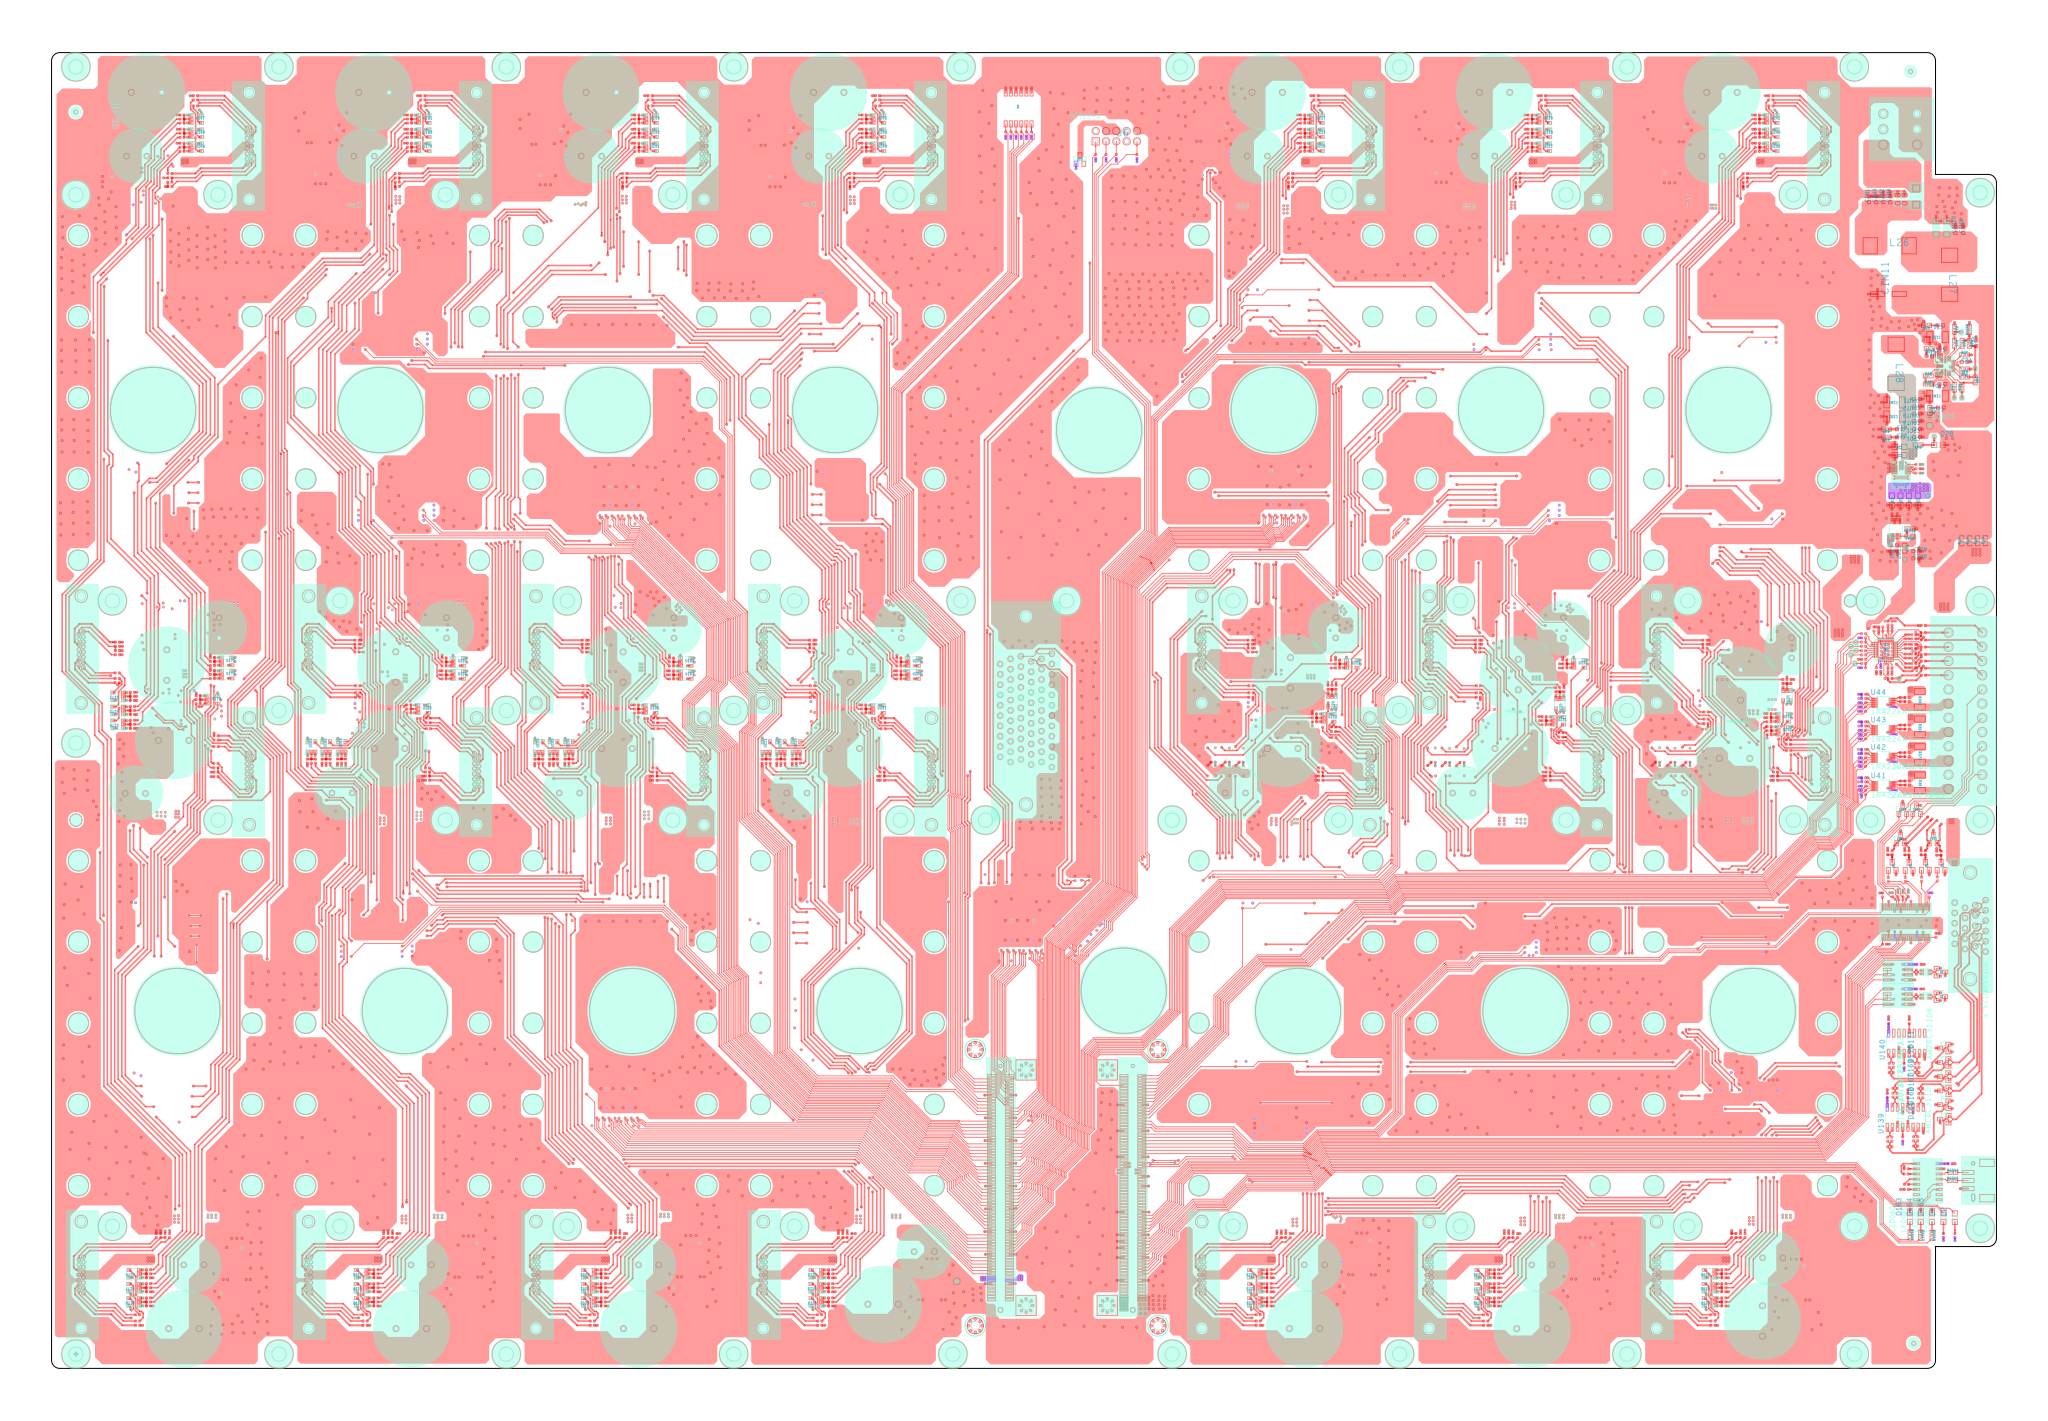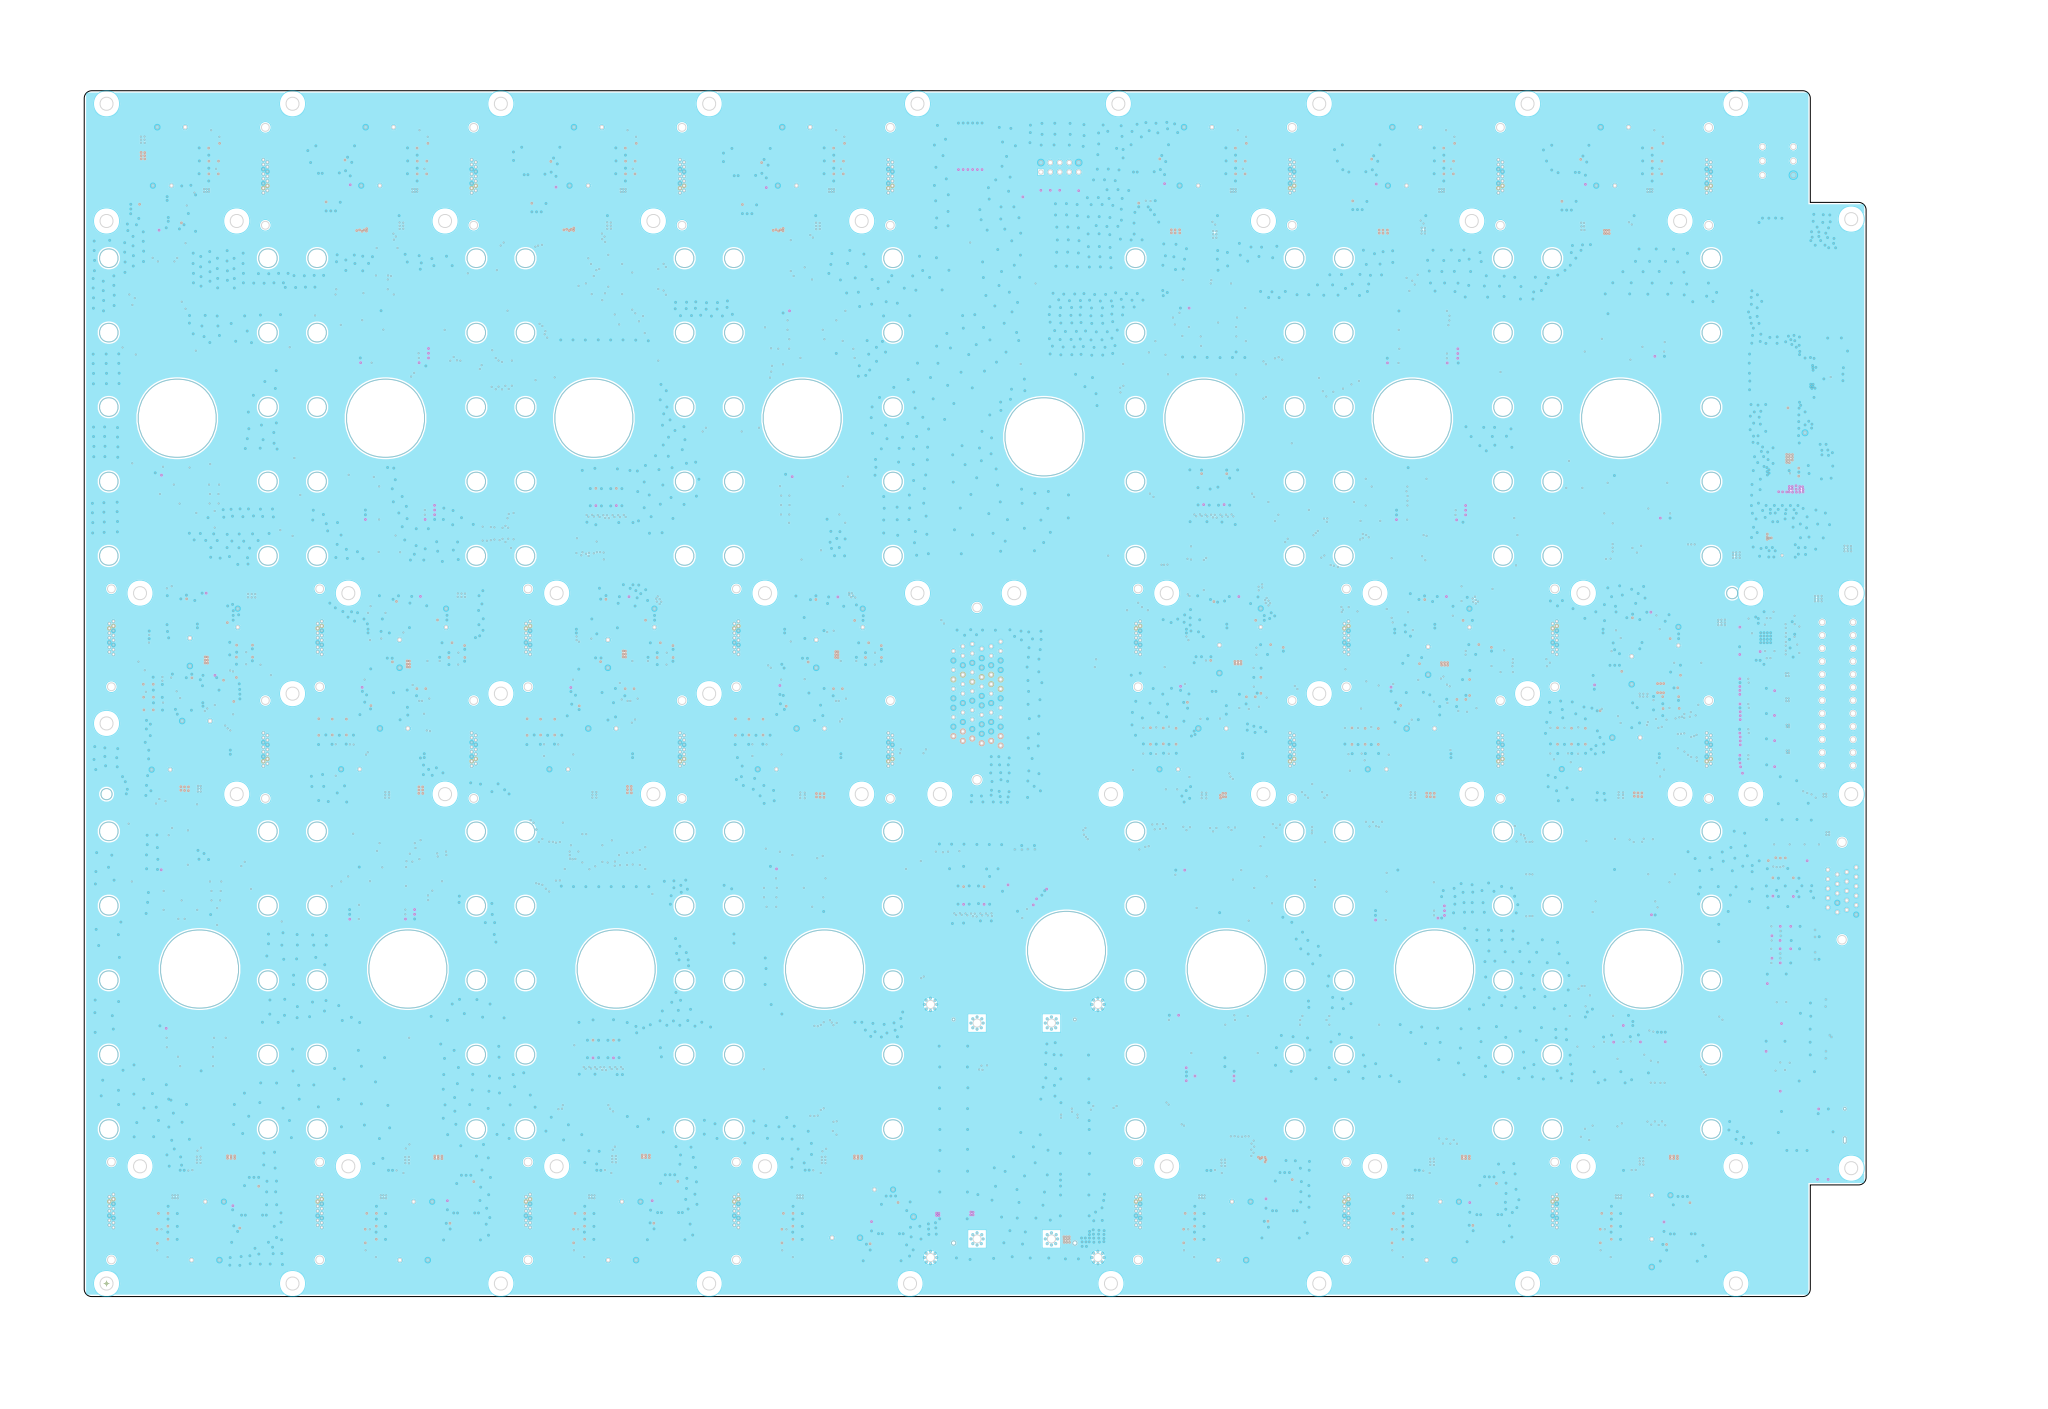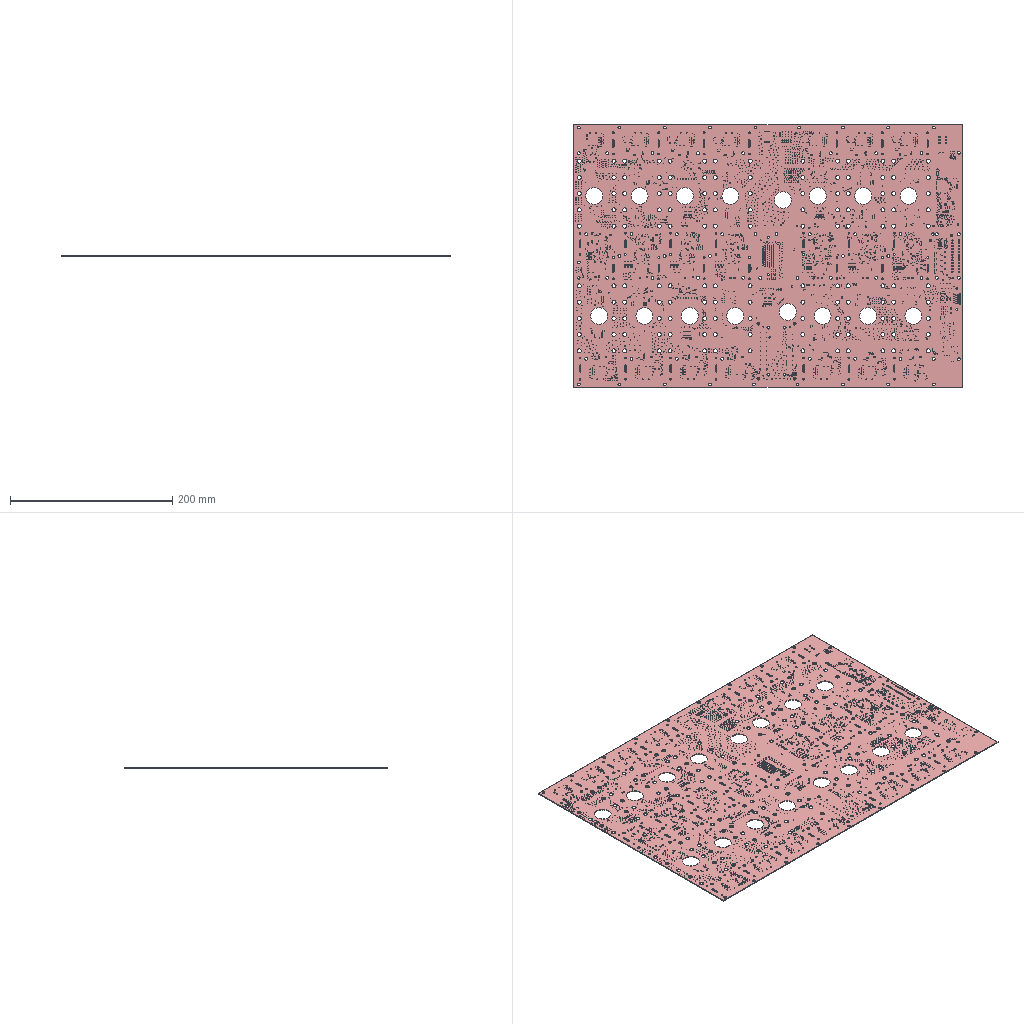Circuit board layout | Cadence Allegro | box 479 x 324 x 1.1 mm
Layer stack:
# Cadence Allegro layer stack of  (unit mm; from the constraint file cross-section; dielectric type: 0 not recorded (Allegro does not mark core vs prepreg), 3 surface material)
index,name,kind,layer,copper_thickness_mm,dielectric_type,dielectric_thickness_mm,dielectric_material,dielectric_constant
0,Top Surface,other,,,,,,
1,TOP,copper,TOP,0.0305,,,,
2,Dielectric1,dielectric,,,0,0.2032,FR-4,4.5
3,GND2,copper,GND2,0.0305,,,,
4,Dielectric2,dielectric,,,0,0.2032,FR-4,4.5
5,POWER3,copper,POWER3,0.0305,,,,
6,Dielectric3,dielectric,,,0,0.2032,FR-4,4.5
7,POWER4,copper,POWER4,0.0305,,,,
8,Dielectric4,dielectric,,,0,0.2032,FR-4,4.5
9,POWER5,copper,POWER5,0.0305,,,,
10,Dielectric5,dielectric,,,0,0.2032,FR-4,4.5
11,BOTTOM,copper,BOTTOM,0.0305,,,,
12,Bottom Surface,other,,,,,,
# drill layer pairs: low layer,high layer
drill_pair,TOP,BOTTOM
Part placement, first 377 of 1998 lines:
REFDES,COMP_VALUE,SYM_NAME,SYM_X,SYM_Y,SYM_ROTATE,SYM_MIRROR
C1A1,CAP/1210,1210,18051.339,9290.378,180.000,NO
C1B1,CAP/1210,1210,18050.898,9860.441,180.000,NO
C1C1,CAP/0603,0603C,18126.119,9750.276,180.000,NO
C1D1,CAP/0603,0603C,18125.516,9405.059,180.000,NO
C2A1,CAP/1210,1210,17634.583,9227.370,180.000,NO
C2B1,CAP/1210,1210,17634.839,9091.150,180.000,NO
C2C1,CAP/0603,0603C,17880.040,8969.595,180.000,NO
C2D1,CAP/0603,0603C,17880.284,8891.701,180.000,NO
C1,0.1uF/50V/10%/X7R/C0402,0402,17868.530,3540.996,0.000,NO
C2,0.1uF/50V/10%/X7R/C0402,0402,17870.629,3778.535,0.000,NO
C3,0.1uF/50V/10%/X7R/C0402,0402,9868.984,4088.897,270.000,YES
C18,CAP/0603,0603C,17943.178,9674.260,0.000,NO
C19,CAP/0603,0603C,17657.426,8967.319,0.000,NO
C20,CAP/0603,0603C,18111.154,9176.590,180.000,NO
C21,CAP/0603,0603C,18105.689,9974.244,180.000,NO
C22,CAP/0603,0603C,17657.623,8889.048,0.000,NO
C23,CAP/0603,0603C,18314.106,9495.446,270.000,YES
C24,CAP/0603,0603C,18286.095,9620.170,0.000,NO
C25,CAP/0603,0603C,18425.634,9773.075,90.000,NO
C26,22uF/10V/10%/X5R/C0805,0805,17681.957,8795.307,180.000,NO
C27,22uF/10V/10%/X5R/C0805,0805,17682.335,8715.925,180.000,NO
C28,22uF/10V/10%/X5R/C0805,0805,17859.493,8275.418,270.000,NO
C29,22uF/10V/10%/X5R/C0805,0805,17691.760,8275.906,270.000,NO
C30,22uF/10V/10%/X5R/C0805,0805,17608.689,8276.016,270.000,NO
C31,22uF/10V/10%/X5R/C0805,0805,17774.485,8275.622,270.000,NO
C32,39pF/6.3V/5%/NP0/C0402,0402,17861.079,8583.465,180.000,YES
C33,1uF/16V/10%/X5R/C0402,0402,11474.713,2195.292,180.000,YES
C34,0.1uF/50V/10%/X7R/C0402,0402,11474.670,2238.174,180.000,YES
C35,0.1uF/50V/10%/X7R/C0402,0402,11886.493,2245.548,180.000,YES
C58,0.1uF/50V/10%/X7R/C0402,0402,17611.040,5487.150,270.000,YES
C59,0.1uF/50V/10%/X7R/C0402,0402,17689.004,5536.973,270.000,NO
C60,0.1uF/50V/10%/X7R/C0402,0402,17609.591,5762.355,270.000,YES
C61,0.1uF/50V/10%/X7R/C0402,0402,17687.556,5812.177,270.000,NO
C62,0.1uF/50V/10%/X7R/C0402,0402,17609.985,6029.410,270.000,YES
C63,0.1uF/50V/10%/X7R/C0402,0402,17687.949,6079.233,270.000,NO
C64,0.1uF/50V/10%/X7R/C0402,0402,17609.725,6296.347,270.000,YES
C65,0.1uF/50V/10%/X7R/C0402,0402,17687.689,6346.170,270.000,NO
C66,0.1uF/50V/10%/X7R/C0402,0402,17832.535,4336.033,180.000,YES
C67,0.1uF/50V/10%/X7R/C0402,0402,17616.252,4336.100,180.000,YES
C68,0.1uF/50V/10%/X7R/C0402,0402,17871.713,4121.929,0.000,YES
C69,0.1uF/50V/10%/X7R/C0402,0402,17655.575,4130.386,0.000,YES
C70,10nF/50V/10%/X7R/C0402,0402,17569.166,6571.114,90.000,YES
C71,0.1uF/50V/10%/X7R/C0402,0402,17589.851,6651.284,0.000,NO
C72,10nF/50V/10%/X7R/C0402,0402,17608.749,6570.331,90.000,YES
C73,0.1uF/50V/10%/X7R/C0402,0402,17466.623,6878.855,180.000,YES
C74,1uF/50V/10%/X7R/C0402,0402,17466.563,6838.792,180.000,YES
C75,0.1uF/50V/10%/X7R/C0402,0402,17500.595,7009.626,180.000,NO
C76,1uF/50V/10%/X7R/C0402,0402,17500.434,7050.618,180.000,NO
C77,10nF/50V/10%/X7R/C0402,0402,17819.402,6655.437,180.000,YES
C78,0.1uF/50V/10%/X7R/C0402,0402,17740.811,6675.335,90.000,NO
C79,10nF/50V/10%/X7R/C0402,0402,17820.189,6695.020,180.000,YES
C80,0.1uF/50V/10%/X7R/C0402,0402,17434.701,7030.992,90.000,NO
C81,0.1uF/50V/10%/X7R/C0402,0402,17458.560,6636.788,270.000,NO
C82,0.1uF/50V/10%/X7R/C0402,0402,17500.536,6637.268,270.000,NO
C83,1uF/50V/10%/X7R/C0402,0402,17520.130,6735.174,180.000,YES
C84,10nF/50V/10%/X7R/C0402,0402,17819.402,6747.957,180.000,YES
C85,0.1uF/50V/10%/X7R/C0402,0402,17740.418,6767.855,90.000,NO
C86,10nF/50V/10%/X7R/C0402,0402,17820.189,6787.540,180.000,YES
C87,10nF/50V/10%/X7R/C0402,0402,17819.796,6935.359,180.000,YES
C88,0.1uF/50V/10%/X7R/C0402,0402,17741.205,6955.256,90.000,NO
C89,10nF/50V/10%/X7R/C0402,0402,17820.189,6975.339,180.000,YES
C92,10nF/50V/10%/X7R/C0402,0402,17610.252,7086.657,270.000,YES
C93,0.1uF/50V/10%/X7R/C0402,0402,17590.386,7009.756,180.000,NO
C94,10nF/50V/10%/X7R/C0402,0402,17570.705,7086.994,270.000,YES
C95,0.1uF/50V/10%/X7R/C0402,0402,17740.418,6861.953,90.000,NO
C96,10nF/50V/10%/X7R/C0402,0402,17818.615,6842.051,180.000,YES
C97,10nF/50V/10%/X7R/C0402,0402,17818.615,6881.658,0.000,NO
C601,0.1uF/50V/10%/X7R/C0402,0402,18173.497,1846.571,0.000,NO
C602,0.1uF/50V/10%/X7R/C0402,0402,17746.798,1746.865,0.000,NO
C603,0.1uF/50V/10%/X7R/C0402,0402,17746.540,1796.941,180.000,NO
C604,0.1uF/50V/10%/X7R/C0402,0402,17748.642,1597.272,0.000,NO
C605,0.1uF/50V/10%/X7R/C0402,0402,17749.111,1646.658,0.000,NO
C779,10uF/10V/10%/X5R/C0603,0603C,17817.149,7784.147,0.000,NO
C780,0.1uF/50V/10%/X7R/C0603,0603C,17817.149,7715.639,0.000,NO
C791,1uF/25V/10%/X7R/C0603,0603C,17595.103,7840.532,270.000,NO
C792,1uF/25V/10%/X7R/C0603,0603C,17660.071,7840.736,270.000,NO
C793,0.1uF/50V/10%/X7R/C0402,0402,17564.020,2508.112,90.000,NO
C794,0.1uF/50V/10%/X7R/C0402,0402,17576.301,3223.981,90.000,NO
C795,0.1uF/50V/10%/X7R/C0402,0402,16496.414,2609.012,270.000,YES
C796,0.1uF/50V/10%/X7R/C0402,0402,16233.607,2610.319,270.000,YES
C797,0.1uF/50V/10%/X7R/C0402,0402,15950.103,2608.174,270.000,YES
C798,0.1uF/50V/10%/X7R/C0402,0402,16105.874,2729.662,180.000,YES
C799,0.1uF/50V/10%/X7R/C0402,0402,558.788,4353.280,0.000,YES
C800,0.1uF/50V/10%/X7R/C0402,0402,584.410,2699.823,0.000,YES
C801,0.1uF/50V/10%/X7R/C0402,0402,534.906,8551.941,0.000,YES
C802,0.1uF/50V/10%/X7R/C0402,0402,7046.056,4386.111,0.000,YES
C803,0.1uF/50V/10%/X7R/C0402,0402,7179.477,10289.481,0.000,YES
C804,0.1uF/50V/10%/X7R/C0402,0402,7206.414,8535.630,0.000,YES
C805,0.1uF/50V/10%/X7R/C0402,0402,11407.186,10319.126,0.000,YES
C806,0.1uF/50V/10%/X7R/C0402,0402,11366.024,4373.528,0.000,YES
C807,0.1uF/50V/10%/X7R/C0402,0402,11295.063,2838.327,0.000,YES
C808,0.1uF/50V/10%/X7R/C0402,0402,16437.414,9808.681,180.000,YES
C809,0.1uF/50V/10%/X7R/C0402,0402,16370.079,3929.650,180.000,YES
C810,0.1uF/50V/10%/X7R/C0402,0402,16497.422,8097.280,180.000,YES
C811,0.1uF/50V/10%/X7R/C0402,0402,3423.780,8082.780,0.000,YES
C812,0.1uF/50V/10%/X7R/C0402,0402,14110.162,3844.087,0.000,YES
C813,0.1uF/50V/10%/X7R/C0402,0402,3211.040,3856.394,0.000,YES
C814,0.1uF/50V/10%/X7R/C0402,0402,14335.974,8080.960,0.000,YES
C815,0.1uF/50V/10%/X7R/C0402,0402,3359.607,9740.831,0.000,YES
C816,0.1uF/50V/10%/X7R/C0402,0402,14254.122,9737.953,0.000,YES
C817,0.1uF/50V/10%/X7R/C0402,0402,5394.308,8577.229,90.000,YES
C818,0.1uF/50V/10%/X7R/C0402,0402,5179.004,8581.733,90.000,YES
C819,0.1uF/50V/10%/X7R/C0402,0402,5394.969,8069.504,270.000,YES
C820,0.1uF/50V/10%/X7R/C0402,0402,5178.331,8073.492,270.000,YES
C821,0.1uF/50V/10%/X7R/C0402,0402,11828.107,8586.008,90.000,YES
C822,0.1uF/50V/10%/X7R/C0402,0402,11611.311,8587.028,90.000,YES
C823,0.1uF/50V/10%/X7R/C0402,0402,11827.276,8074.799,270.000,YES
C824,0.1uF/50V/10%/X7R/C0402,0402,11610.638,8078.788,270.000,YES
C825,0.1uF/50V/10%/X7R/C0402,0402,5365.749,2741.473,90.000,YES
C826,0.1uF/50V/10%/X7R/C0402,0402,5148.953,2742.492,90.000,YES
C827,0.1uF/50V/10%/X7R/C0402,0402,5364.918,2230.264,270.000,YES
C828,0.1uF/50V/10%/X7R/C0402,0402,5148.280,2234.252,270.000,YES
C829,0.1uF/50V/10%/X7R/C0402,0402,9286.972,4365.877,90.000,YES
C830,0.1uF/50V/10%/X7R/C0402,0402,9070.921,4367.893,90.000,YES
C831,0.1uF/50V/10%/X7R/C0402,0402,9070.248,3859.652,270.000,YES
C832,0.1uF/50V/10%/X7R/C0402,0402,9286.886,3855.664,270.000,YES
C833,0.1uF/50V/10%/X7R/C0402,0402,1029.527,11873.502,0.000,YES
C834,0.1uF/50V/10%/X7R/C0402,0402,1028.959,11738.009,0.000,YES
C835,0.1uF/50V/10%/X7R/C0402,0402,1028.945,12011.644,0.000,YES
C836,0.1uF/50V/10%/X7R/C0402,0402,547.436,6202.997,180.000,YES
C837,0.1uF/50V/10%/X7R/C0402,0402,546.904,6339.429,180.000,YES
C838,0.1uF/50V/10%/X7R/C0402,0402,547.436,6068.153,180.000,YES
C839,0.1uF/50V/10%/X7R/C0402,0402,1512.328,6606.945,90.000,YES
C840,0.1uF/50V/10%/X7R/C0402,0402,1374.048,6363.565,90.000,YES
C841,0.1uF/50V/10%/X7R/C0402,0402,1512.196,6733.853,90.000,YES
C842,0.1uF/50V/10%/X7R/C0402,0402,702.697,606.800,180.000,YES
C843,0.1uF/50V/10%/X7R/C0402,0402,703.347,468.846,180.000,YES
C844,0.1uF/50V/10%/X7R/C0402,0402,703.740,742.493,180.000,YES
C845,0.1uF/50V/10%/X7R/C0402,0402,3234.627,11873.502,0.000,YES
C846,0.1uF/50V/10%/X7R/C0402,0402,3234.045,12011.644,0.000,YES
C847,0.1uF/50V/10%/X7R/C0402,0402,3234.059,11738.009,0.000,YES
C848,0.1uF/50V/10%/X7R/C0402,0402,3758.492,6602.981,90.000,YES
C849,0.1uF/50V/10%/X7R/C0402,0402,3315.152,6272.937,90.000,YES
C850,0.1uF/50V/10%/X7R/C0402,0402,3760.076,6728.837,90.000,YES
C851,0.1uF/50V/10%/X7R/C0402,0402,2265.698,5834.736,180.000,YES
C852,0.1uF/50V/10%/X7R/C0402,0402,2408.361,5834.885,180.000,YES
C853,0.1uF/50V/10%/X7R/C0402,0402,2557.991,5835.767,180.000,YES
C854,0.1uF/50V/10%/X7R/C0402,0402,2908.572,742.457,180.000,YES
C855,0.1uF/50V/10%/X7R/C0402,0402,2907.529,606.764,180.000,YES
C856,0.1uF/50V/10%/X7R/C0402,0402,2908.179,468.810,180.000,YES
C857,0.1uF/50V/10%/X7R/C0402,0402,5439.207,11873.514,0.000,YES
C858,0.1uF/50V/10%/X7R/C0402,0402,5438.625,12011.656,0.000,YES
C859,0.1uF/50V/10%/X7R/C0402,0402,5438.639,11738.021,0.000,YES
C860,0.1uF/50V/10%/X7R/C0402,0402,4762.715,5835.275,180.000,YES
C861,0.1uF/50V/10%/X7R/C0402,0402,5519.876,6272.445,90.000,YES
C862,0.1uF/50V/10%/X7R/C0402,0402,4470.422,5834.244,180.000,YES
C863,0.1uF/50V/10%/X7R/C0402,0402,5963.216,6602.489,90.000,YES
C864,0.1uF/50V/10%/X7R/C0402,0402,4613.085,5834.393,180.000,YES
C865,0.1uF/50V/10%/X7R/C0402,0402,5964.800,6728.345,90.000,YES
C866,0.1uF/50V/10%/X7R/C0402,0402,5112.097,606.772,180.000,YES
C867,0.1uF/50V/10%/X7R/C0402,0402,5113.140,742.465,180.000,YES
C868,0.1uF/50V/10%/X7R/C0402,0402,5112.747,468.818,180.000,YES
C869,0.1uF/50V/10%/X7R/C0402,0402,7643.211,11738.021,0.000,YES
C870,0.1uF/50V/10%/X7R/C0402,0402,7643.779,11873.514,0.000,YES
C871,0.1uF/50V/10%/X7R/C0402,0402,7643.197,12011.656,0.000,YES
C872,0.1uF/50V/10%/X7R/C0402,0402,6967.435,5835.287,180.000,YES
C873,0.1uF/50V/10%/X7R/C0402,0402,6675.142,5834.256,180.000,YES
C874,0.1uF/50V/10%/X7R/C0402,0402,7724.596,6272.457,90.000,YES
C875,0.1uF/50V/10%/X7R/C0402,0402,8167.936,6602.501,90.000,YES
C876,0.1uF/50V/10%/X7R/C0402,0402,8169.520,6728.357,90.000,YES
C877,0.1uF/50V/10%/X7R/C0402,0402,6817.805,5834.405,180.000,YES
C878,0.1uF/50V/10%/X7R/C0402,0402,7316.937,606.516,180.000,YES
C879,0.1uF/50V/10%/X7R/C0402,0402,7317.587,468.562,180.000,YES
C880,0.1uF/50V/10%/X7R/C0402,0402,7317.980,742.209,180.000,YES
C881,0.1uF/50V/10%/X7R/C0402,0402,11895.299,11738.033,0.000,YES
C882,0.1uF/50V/10%/X7R/C0402,0402,11895.867,11873.526,0.000,YES
C883,0.1uF/50V/10%/X7R/C0402,0402,11895.285,12011.668,0.000,YES
C884,0.1uF/50V/10%/X7R/C0402,0402,12094.660,6186.713,90.000,YES
C885,0.1uF/50V/10%/X7R/C0402,0402,12196.924,6277.117,0.000,YES
C886,0.1uF/50V/10%/X7R/C0402,0402,11299.425,5738.603,180.000,NO
C887,0.1uF/50V/10%/X7R/C0402,0402,12423.692,6709.069,90.000,YES
C888,0.1uF/50V/10%/X7R/C0402,0402,11028.474,5739.592,180.000,NO
C889,0.1uF/50V/10%/X7R/C0402,0402,11164.603,5740.557,180.000,NO
C890,0.1uF/50V/10%/X7R/C0402,0402,11569.804,742.485,180.000,YES
C891,0.1uF/50V/10%/X7R/C0402,0402,11568.761,606.792,180.000,YES
C892,0.1uF/50V/10%/X7R/C0402,0402,11569.411,468.838,180.000,YES
C893,0.1uF/50V/10%/X7R/C0402,0402,14100.443,11873.534,0.000,YES
C894,0.1uF/50V/10%/X7R/C0402,0402,14099.875,11738.041,0.000,YES
C895,0.1uF/50V/10%/X7R/C0402,0402,14099.861,12011.676,0.000,YES
C896,0.1uF/50V/10%/X7R/C0402,0402,13161.162,5738.004,180.000,NO
C897,0.1uF/50V/10%/X7R/C0402,0402,14626.800,6709.717,90.000,YES
C898,0.1uF/50V/10%/X7R/C0402,0402,13300.527,5736.537,180.000,NO
C899,0.1uF/50V/10%/X7R/C0402,0402,13440.225,5736.203,180.000,NO
C900,0.1uF/50V/10%/X7R/C0402,0402,14322.484,6158.993,90.000,YES
C901,0.1uF/50V/10%/X7R/C0402,0402,14406.000,6253.705,0.000,YES
C902,0.1uF/50V/10%/X7R/C0402,0402,13774.504,742.229,180.000,YES
C903,0.1uF/50V/10%/X7R/C0402,0402,13773.461,606.536,180.000,YES
C904,0.1uF/50V/10%/X7R/C0402,0402,13774.111,468.582,180.000,YES
C905,0.1uF/50V/10%/X7R/C0402,0402,16305.271,11873.270,0.000,YES
C906,0.1uF/50V/10%/X7R/C0402,0402,16304.689,12011.412,0.000,YES
C907,0.1uF/50V/10%/X7R/C0402,0402,16304.703,11737.777,0.000,YES
C908,0.1uF/50V/10%/X7R/C0402,0402,15485.059,5738.173,180.000,NO
C909,0.1uF/50V/10%/X7R/C0402,0402,16608.108,6331.565,0.000,YES
C910,0.1uF/50V/10%/X7R/C0402,0402,15336.774,5739.640,180.000,NO
C911,0.1uF/50V/10%/X7R/C0402,0402,15631.237,5738.651,180.000,NO
C912,0.1uF/50V/10%/X7R/C0402,0402,16504.268,6062.561,90.000,YES
C913,0.1uF/50V/10%/X7R/C0402,0402,16605.204,6188.377,90.000,YES
C914,0.1uF/50V/10%/X7R/C0402,0402,15978.033,606.812,180.000,YES
C915,0.1uF/50V/10%/X7R/C0402,0402,15979.076,742.505,180.000,YES
C916,0.1uF/50V/10%/X7R/C0402,0402,15978.683,468.858,180.000,YES
C917,0.1uF/50V/10%/X7R/C0402,0402,792.932,11175.945,90.000,YES
C918,2pF/50V/10%/X7R/C0402,0402,699.080,11236.993,0.000,YES
C919,2pF/50V/10%/X7R/C0402,0402,699.864,11497.509,0.000,YES
C920,0.1uF/50V/10%/X7R/C0402,0402,304.672,11416.841,0.000,YES
C921,0.1uF/50V/10%/X7R/C0402,0402,820.324,7262.541,270.000,YES
C922,0.1uF/50V/10%/X7R/C0402,0402,1298.048,7017.737,180.000,YES
C923,2pF/50V/10%/X7R/C0402,0402,914.176,7196.773,180.000,YES
C924,2pF/50V/10%/X7R/C0402,0402,913.392,6937.069,180.000,YES
C925,0.1uF/50V/10%/X7R/C0402,0402,878.988,6426.733,270.000,YES
C926,0.1uF/50V/10%/X7R/C0402,0402,1366.688,586.357,0.000,YES
C927,0.1uF/50V/10%/X7R/C0402,0402,1609.904,1073.401,270.000,YES
C928,2pF/50V/10%/X7R/C0402,0402,1429.100,679.529,270.000,YES
C929,2pF/50V/10%/X7R/C0402,0402,1690.976,679.425,270.000,YES
C930,0.1uF/50V/10%/X7R/C0402,0402,1366.204,6184.709,180.000,YES
C931,2pF/50V/10%/X7R/C0402,0402,972.672,6363.985,180.000,YES
C932,2pF/50V/10%/X7R/C0402,0402,971.888,6104.149,180.000,YES
C933,0.1uF/50V/10%/X7R/C0402,0402,2575.444,11885.253,180.000,YES
C934,0.1uF/50V/10%/X7R/C0402,0402,3547.896,7019.189,180.000,YES
C935,0.1uF/50V/10%/X7R/C0402,0402,3068.684,7255.697,270.000,YES
C936,2pF/50V/10%/X7R/C0402,0402,3162.536,7198.093,180.000,YES
C937,2pF/50V/10%/X7R/C0402,0402,3161.752,6938.389,180.000,YES
C938,0.1uF/50V/10%/X7R/C0402,0402,2752.284,6113.205,0.000,YES
C939,0.1uF/50V/10%/X7R/C0402,0402,3614.840,610.869,0.000,YES
C940,0.1uF/50V/10%/X7R/C0402,0402,3855.332,1097.913,270.000,YES
C941,2pF/50V/10%/X7R/C0402,0402,3674.528,704.721,270.000,YES
C942,2pF/50V/10%/X7R/C0402,0402,3936.404,703.937,270.000,YES
C943,0.1uF/50V/10%/X7R/C0402,0402,2996.244,6595.385,270.000,YES
C944,2pF/50V/10%/X7R/C0402,0402,2816.396,6207.057,270.000,YES
C945,2pF/50V/10%/X7R/C0402,0402,3076.912,6206.273,270.000,YES
C946,0.1uF/50V/10%/X7R/C0402,0402,2323.768,11397.777,90.000,YES
C947,2pF/50V/10%/X7R/C0402,0402,2503.460,11791.217,90.000,YES
C948,2pF/50V/10%/X7R/C0402,0402,2242.944,11792.001,90.000,YES
C949,0.1uF/50V/10%/X7R/C0402,0402,4750.732,11870.145,180.000,YES
C950,0.1uF/50V/10%/X7R/C0402,0402,5750.384,7017.469,180.000,YES
C951,0.1uF/50V/10%/X7R/C0402,0402,5263.340,7257.961,270.000,YES
C952,2pF/50V/10%/X7R/C0402,0402,5357.192,7195.889,180.000,YES
C953,2pF/50V/10%/X7R/C0402,0402,5356.408,6936.397,180.000,YES
C954,0.1uF/50V/10%/X7R/C0402,0402,4962.176,6110.765,0.000,YES
C955,0.1uF/50V/10%/X7R/C0402,0402,5772.196,612.489,0.000,YES
C956,0.1uF/50V/10%/X7R/C0402,0402,6013.200,1100.385,270.000,YES
C957,2pF/50V/10%/X7R/C0402,0402,5832.564,706.341,270.000,YES
C958,2pF/50V/10%/X7R/C0402,0402,6093.760,705.557,270.000,YES
C959,0.1uF/50V/10%/X7R/C0402,0402,5202.668,6597.809,270.000,YES
C960,2pF/50V/10%/X7R/C0402,0402,5024.584,6203.937,270.000,YES
C961,2pF/50V/10%/X7R/C0402,0402,5283.740,6203.833,270.000,YES
C962,0.1uF/50V/10%/X7R/C0402,0402,4501.228,11383.441,90.000,YES
C963,2pF/50V/10%/X7R/C0402,0402,4679.988,11776.633,90.000,YES
C964,2pF/50V/10%/X7R/C0402,0402,4420.156,11777.417,90.000,YES
C965,0.1uF/50V/10%/X7R/C0402,0402,6729.612,11366.449,90.000,YES
C966,0.1uF/50V/10%/X7R/C0402,0402,7479.868,7255.525,270.000,YES
C967,0.1uF/50V/10%/X7R/C0402,0402,7962.860,7015.033,180.000,YES
C968,2pF/50V/10%/X7R/C0402,0402,7571.168,7193.793,180.000,YES
C969,2pF/50V/10%/X7R/C0402,0402,7572.764,6933.449,180.000,YES
C970,0.1uF/50V/10%/X7R/C0402,0402,7392.028,6594.201,270.000,YES
C971,0.1uF/50V/10%/X7R/C0402,0402,8350.832,876.805,270.000,YES
C972,0.1uF/50V/10%/X7R/C0402,0402,8061.516,390.441,0.000,YES
C973,2pF/50V/10%/X7R/C0402,0402,8169.856,482.593,270.000,YES
C974,2pF/50V/10%/X7R/C0402,0402,8431.392,482.149,270.000,YES
C975,0.1uF/50V/10%/X7R/C0402,0402,7151.536,6107.157,0.000,YES
C976,2pF/50V/10%/X7R/C0402,0402,7213.604,6201.353,270.000,YES
C977,2pF/50V/10%/X7R/C0402,0402,7473.100,6200.225,270.000,YES
C978,0.1uF/50V/10%/X7R/C0402,0402,6981.676,11857.917,180.000,YES
C979,2pF/50V/10%/X7R/C0402,0402,6909.740,11764.065,90.000,YES
C980,2pF/50V/10%/X7R/C0402,0402,6643.100,11764.849,90.000,YES
C981,0.1uF/50V/10%/X7R/C0402,0402,11189.860,11896.821,180.000,YES
C982,0.1uF/50V/10%/X7R/C0402,0402,11739.332,7236.017,180.000,YES
C983,0.1uF/50V/10%/X7R/C0402,0402,12207.984,7015.977,180.000,YES
C984,2pF/50V/10%/X7R/C0402,0402,11813.088,7196.101,180.000,YES
C985,2pF/50V/10%/X7R/C0402,0402,11812.304,6935.585,180.000,YES
C986,0.1uF/50V/10%/X7R/C0402,0402,11662.736,6611.225,270.000,YES
C987,0.1uF/50V/10%/X7R/C0402,0402,12272.164,632.629,0.000,YES
C988,0.1uF/50V/10%/X7R/C0402,0402,12518.780,1118.993,270.000,YES
C989,2pF/50V/10%/X7R/C0402,0402,12340.696,726.821,270.000,YES
C990,2pF/50V/10%/X7R/C0402,0402,12599.852,725.017,270.000,YES
C991,0.1uF/50V/10%/X7R/C0402,0402,11419.528,6123.161,0.000,YES
C992,2pF/50V/10%/X7R/C0402,0402,11480.576,6217.013,270.000,YES
C993,2pF/50V/10%/X7R/C0402,0402,11741.092,6216.229,270.000,YES
C994,0.1uF/50V/10%/X7R/C0402,0402,10949.368,11409.777,90.000,YES
C995,2pF/50V/10%/X7R/C0402,0402,11127.796,11803.649,90.000,YES
C996,2pF/50V/10%/X7R/C0402,0402,10868.296,11803.753,90.000,YES
C997,0.1uF/50V/10%/X7R/C0402,0402,13433.856,11894.801,180.000,YES
C998,0.1uF/50V/10%/X7R/C0402,0402,14403.352,7015.037,180.000,YES
C999,0.1uF/50V/10%/X7R/C0402,0402,13924.412,7254.717,270.000,YES
C1000,2pF/50V/10%/X7R/C0402,0402,14014.212,7193.801,180.000,YES
C1001,2pF/50V/10%/X7R/C0402,0402,14013.832,6933.965,180.000,YES
C1002,0.1uF/50V/10%/X7R/C0402,0402,13894.836,6601.701,270.000,YES
C1003,0.1uF/50V/10%/X7R/C0402,0402,14683.836,1079.149,270.000,YES
C1004,0.1uF/50V/10%/X7R/C0402,0402,14440.964,591.425,0.000,YES
C1005,2pF/50V/10%/X7R/C0402,0402,14502.696,685.277,270.000,YES
C1006,2pF/50V/10%/X7R/C0402,0402,14764.908,684.493,270.000,YES
C1007,0.1uF/50V/10%/X7R/C0402,0402,13654.344,6114.657,0.000,YES
C1008,2pF/50V/10%/X7R/C0402,0402,13715.392,6208.509,270.000,YES
C1009,2pF/50V/10%/X7R/C0402,0402,13975.908,6207.725,270.000,YES
C1010,0.1uF/50V/10%/X7R/C0402,0402,13189.384,11408.165,90.000,YES
C1011,2pF/50V/10%/X7R/C0402,0402,13367.812,11801.357,90.000,YES
C1012,2pF/50V/10%/X7R/C0402,0402,13108.312,11802.141,90.000,YES
C1013,0.1uF/50V/10%/X7R/C0402,0402,15402.788,11404.073,90.000,YES
C1014,0.1uF/50V/10%/X7R/C0402,0402,16125.148,7061.833,270.000,YES
C1015,0.1uF/50V/10%/X7R/C0402,0402,16593.956,6822.149,180.000,YES
C1016,2pF/50V/10%/X7R/C0402,0402,16207.248,7000.573,180.000,YES
C1017,2pF/50V/10%/X7R/C0402,0402,16207.276,6741.481,180.000,YES
C1018,0.1uF/50V/10%/X7R/C0402,0402,16036.216,6520.621,270.000,YES
C1019,0.1uF/50V/10%/X7R/C0402,0402,16490.472,386.793,0.000,YES
C1020,0.1uF/50V/10%/X7R/C0402,0402,16731.304,874.517,270.000,YES
C1021,2pF/50V/10%/X7R/C0402,0402,16551.520,480.645,270.000,YES
C1022,2pF/50V/10%/X7R/C0402,0402,16812.036,479.861,270.000,YES
C1023,0.1uF/50V/10%/X7R/C0402,0402,15795.384,6029.833,0.000,YES
C1024,2pF/50V/10%/X7R/C0402,0402,15856.432,6123.685,270.000,YES
C1025,2pF/50V/10%/X7R/C0402,0402,16116.948,6122.901,270.000,YES
C1026,0.1uF/50V/10%/X7R/C0402,0402,15645.652,11891.965,180.000,YES
C1027,2pF/50V/10%/X7R/C0402,0402,15584.940,11799.469,90.000,YES
C1028,2pF/50V/10%/X7R/C0402,0402,15322.392,11798.897,90.000,YES
C1029,10nF/50V/10%/X7R/C0402,0402,17616.296,4454.445,270.000,YES
C1030,10nF/50V/10%/X7R/C0402,0402,17665.668,4454.113,270.000,YES
C1031,10nF/50V/10%/X7R/C0402,0402,17714.552,4453.949,270.000,YES
C1032,10nF/50V/10%/X7R/C0402,0402,17767.548,4454.605,270.000,YES
CIN1,CAP/0603,0603C,17385.702,11168.511,90.000,NO
CIN2,CAP/0603,0603C,17525.548,11168.740,90.000,NO
CIN3,CAP/0603,0603C,17457.580,11168.866,90.000,NO
CIN4,CAP/0603,0603C,17592.757,11168.948,90.000,NO
CIN5,CAP/0603,0805C,17664.422,11196.650,90.000,NO
CIN6,CAP/0603,0805C,17730.831,11195.469,90.000,NO
CIN7,CAP/0603,1206,18141.174,10920.569,90.000,NO
CIN8,CAP/0603,1206,18037.183,10919.912,90.000,NO
CIN9,CAP/0603,0603C,18299.544,10870.094,90.000,NO
CIN10,CAP/0603,0603C,18226.162,10869.386,90.000,NO
CIN11,CAP/ELECT/DIP/OD5.3P2.0,AP-SMD_BD6_3-L6_6-W6_6-LS7_21,17574.311,10277.788,180.000,NO
CIN12,ECF1HM182M27OTPO,AP-SMD_BD18-L27-W6_6-LS7_21,684.709,12232.603,270.000,NO
CIN13,ECF1JM331G20OTPO,AP-SMD_BD10-L20-W6_6-LS7_21,588.772,11614.355,270.000,NO
CIN14,ECF1HM182M27OTPO,AP-SMD_BD18-L27-W6_6-LS7_21,881.914,6680.307,0.000,NO
CIN15,ECF1JM331G20OTPO,AP-SMD_BD10-L20-W6_6-LS7_21,1388.626,7040.910,180.000,NO
CIN16,ECF1HM182M27OTPO,AP-SMD_BD18-L27-W6_6-LS7_21,947.788,5950.744,270.000,NO
CIN17,ECF1JM331G20OTPO,AP-SMD_BD10-L20-W6_6-LS7_21,575.662,5436.268,270.000,NO
CIN18,ECF1HM182M27OTPO,AP-SMD_BD18-L27-W6_6-LS7_21,1047.351,247.831,90.000,NO
CIN19,ECF1JM331G20OTPO,AP-SMD_BD10-L20-W6_6-LS7_21,1143.288,866.079,90.000,NO
CIN20,ECF1HM182M27OTPO,AP-SMD_BD18-L27-W6_6-LS7_21,2889.809,12232.603,270.000,NO
CIN21,ECF1JM331G20OTPO,AP-SMD_BD10-L20-W6_6-LS7_21,2793.872,11614.355,270.000,NO
CIN22,ECF1HM182M27OTPO,AP-SMD_BD18-L27-W6_6-LS7_21,3101.180,6661.813,0.000,NO
CIN23,ECF1JM331G20OTPO,AP-SMD_BD10-L20-W6_6-LS7_21,3593.540,7041.044,180.000,NO
CIN24,ECF1JM331G20OTPO,AP-SMD_BD10-L20-W6_6-LS7_21,2580.835,5440.351,270.000,NO
CIN25,ECF1HM182M27OTPO,AP-SMD_BD18-L27-W6_6-LS7_21,3041.012,5872.040,270.000,NO
CIN26,ECF1HM182M27OTPO,AP-SMD_BD18-L27-W6_6-LS7_21,3252.183,247.795,90.000,NO
CIN27,ECF1JM331G20OTPO,AP-SMD_BD10-L20-W6_6-LS7_21,3348.120,866.043,90.000,NO
CIN28,ECF1HM182M27OTPO,AP-SMD_BD18-L27-W6_6-LS7_21,5094.389,12232.615,270.000,NO
CIN29,ECF1JM331G20OTPO,AP-SMD_BD10-L20-W6_6-LS7_21,4998.452,11614.367,270.000,NO
CIN30,ECF1HM182M27OTPO,AP-SMD_BD18-L27-W6_6-LS7_21,5305.904,6661.321,0.000,NO
CIN31,ECF1JM331G20OTPO,AP-SMD_BD10-L20-W6_6-LS7_21,5798.264,7040.552,180.000,NO
CIN32,ECF1HM182M27OTPO,AP-SMD_BD18-L27-W6_6-LS7_21,5245.736,5871.548,270.000,NO
CIN33,ECF1JM331G20OTPO,AP-SMD_BD10-L20-W6_6-LS7_21,4785.559,5439.859,270.000,NO
CIN34,ECF1HM182M27OTPO,AP-SMD_BD18-L27-W6_6-LS7_21,5456.751,247.803,90.000,NO
CIN35,ECF1JM331G20OTPO,AP-SMD_BD10-L20-W6_6-LS7_21,5552.688,866.051,90.000,NO
CIN36,ECF1HM182M27OTPO,AP-SMD_BD18-L27-W6_6-LS7_21,7298.961,12232.615,270.000,NO
CIN37,ECF1JM331G20OTPO,AP-SMD_BD10-L20-W6_6-LS7_21,7203.024,11614.367,270.000,NO
CIN38,ECF1JM331G20OTPO,AP-SMD_BD10-L20-W6_6-LS7_21,6990.279,5439.871,270.000,NO
CIN39,ECF1HM182M27OTPO,AP-SMD_BD18-L27-W6_6-LS7_21,7450.456,5871.560,270.000,NO
CIN40,ECF1JM331G20OTPO,AP-SMD_BD10-L20-W6_6-LS7_21,8002.984,7040.564,180.000,NO
CIN41,ECF1HM182M27OTPO,AP-SMD_BD18-L27-W6_6-LS7_21,7510.624,6661.333,0.000,NO
CIN42,ECF1HM182M27OTPO,AP-SMD_BD18-L27-W6_6-LS7_21,7826.575,484.451,90.000,NO
CIN43,ECF1JM331G20OTPO,AP-SMD_BD10-L20-W6_6-LS7_21,8225.584,994.083,90.000,NO
CIN44,ECF1HM182M27OTPO,AP-SMD_BD18-L27-W6_6-LS7_21,11551.049,12232.627,270.000,NO
CIN45,ECF1JM331G20OTPO,AP-SMD_BD10-L20-W6_6-LS7_21,11455.112,11614.379,270.000,NO
CIN46,ECF1HM182M27OTPO,AP-SMD_BD18-L27-W6_6-LS7_21,11777.764,6605.569,0.000,NO
CIN47,ECF1JM331G20OTPO,AP-SMD_BD10-L20-W6_6-LS7_21,12215.016,7042.344,180.000,NO
CIN48,ECF1HM182M27OTPO,AP-SMD_BD18-L27-W6_6-LS7_21,11702.196,5871.720,270.000,NO
CIN49,ECF1JM331G20OTPO,AP-SMD_BD10-L20-W6_6-LS7_21,11242.019,5440.031,270.000,NO
CIN50,ECF1HM182M27OTPO,AP-SMD_BD18-L27-W6_6-LS7_21,11913.415,247.823,90.000,NO
CIN51,ECF1JM331G20OTPO,AP-SMD_BD10-L20-W6_6-LS7_21,12009.352,866.071,90.000,NO
CIN52,ECF1JM331G20OTPO,AP-SMD_BD10-L20-W6_6-LS7_21,13659.688,11614.387,270.000,NO
CIN53,ECF1HM182M27OTPO,AP-SMD_BD18-L27-W6_6-LS7_21,13755.625,12232.635,270.000,NO
CIN54,ECF1JM331G20OTPO,AP-SMD_BD10-L20-W6_6-LS7_21,13446.747,5439.871,270.000,NO
CIN55,ECF1HM182M27OTPO,AP-SMD_BD18-L27-W6_6-LS7_21,13906.924,5871.560,270.000,NO
CIN56,ECF1HM182M27OTPO,AP-SMD_BD18-L27-W6_6-LS7_21,13986.544,6588.393,0.000,NO
CIN57,ECF1JM331G20OTPO,AP-SMD_BD10-L20-W6_6-LS7_21,14423.792,7040.564,180.000,NO
CIN58,ECF1HM182M27OTPO,AP-SMD_BD18-L27-W6_6-LS7_21,14118.115,247.567,90.000,NO
CIN59,ECF1JM331G20OTPO,AP-SMD_BD10-L20-W6_6-LS7_21,14214.052,865.815,90.000,NO
CIN60,ECF1HM182M27OTPO,AP-SMD_BD18-L27-W6_6-LS7_21,15960.453,12232.371,270.000,NO
Pad and via stacks, first 109 of 124 lines:
# Allegro (Cadence) via spans and padstacks; design units: ("mils" 3 1000)
# via spans: padstack,start_layer,end_layer,net_example,count
VIA12X20,ETCH/TOP,ETCH/BOTTOM,AGND,4791
VIA12X20,ETCH/BOTTOM,ETCH/TOP,AGND,40
# Allegro padstack definitions: name,start_layer,end_layer,drill,plating,holeType,type
2020B,"ETCH/TOP","ETCH/TOP",0.0,"PLATED","none","smd"
SMD_R551X500P0S40,"ETCH/TOP","ETCH/TOP",0.0,"PLATED","none","smd"
PSM_065X081R,"ETCH/TOP","ETCH/TOP",0.0,"PLATED","none","smd"
SMD50_50,"ETCH/TOP","ETCH/TOP",0.0,"PLATED","none","smd"
SMD200X50,"ETCH/TOP","ETCH/TOP",0.0,"PLATED","none","smd"
R75X85,"ETCH/TOP","ETCH/TOP",0.0,"NON_PLATED","none","smd"
RE55X40,"ETCH/TOP","ETCH/TOP",0.0,"NON_PLATED","none","smd"
SMD_R591X1063P0S40,"ETCH/TOP","ETCH/TOP",0.0,"PLATED","none","smd"
Y10,"ETCH/TOP","ETCH/TOP",0.0,"NON_PLATED","none","smd"
R61X15,"ETCH/TOP","ETCH/TOP",0.0,"NON_PLATED","none","smd"
SMD_S50P0S40,"ETCH/TOP","ETCH/TOP",0.0,"PLATED","none","smd"
SMD_R510X80P0S0,"ETCH/TOP","ETCH/TOP",0.0,"PLATED","none","smd"
SMD_R810X100P0S0,"ETCH/TOP","ETCH/TOP",0.0,"PLATED","none","smd"
S_R197T60D2M197_60P197_60,"ETCH/TOP","ETCH/TOP",0.0,"PLATED","none","smd"
S_R147T28D2M147_28P147_28,"ETCH/TOP","ETCH/TOP",0.0,"PLATED","none","smd"
R150_30_K,"ETCH/TOP","ETCH/TOP",0.0,"NON_PLATED","none","smd"
RX148Y148D0T,"ETCH/TOP","ETCH/TOP",0.0,"PLATED","none","smd"
RX10Y32D0T,"ETCH/TOP","ETCH/TOP",0.0,"PLATED","none","smd"
SMD36_50,"ETCH/TOP","ETCH/TOP",0.0,"PLATED","none","smd"
PSM_091S_PM,"ETCH/TOP","ETCH/TOP",0.0,"NON_PLATED","none","smd"
R105_100,"ETCH/TOP","ETCH/TOP",0.0,"PLATED","none","smd"
BGA10_SMD0X619,"ETCH/TOP","ETCH/TOP",0.0,"NON_PLATED","none","smd"
O0R9X1R4,"ETCH/TOP","ETCH/TOP",0.0,"NON_PLATED","none","smd"
R127X152,"ETCH/TOP","ETCH/TOP",0.0,"NON_PLATED","none","smd"
SMD_R1378X472P0S20,"ETCH/TOP","ETCH/TOP",0.0,"PLATED","none","smd"
SMD_R600X300P0S20,"ETCH/TOP","ETCH/TOP",0.0,"PLATED","none","smd"
SMD_R1378X1575P0S20,"ETCH/TOP","ETCH/TOP",0.0,"PLATED","none","smd"
RX43Y10D0T,"ETCH/TOP","ETCH/TOP",0.0,"PLATED","none","smd"
RX59Y10D0T,"ETCH/TOP","ETCH/TOP",0.0,"PLATED","none","smd"
RX5Y5D0T,"ETCH/TOP","ETCH/TOP",0.0,"PLATED","none","smd"
RX28Y10D0T,"ETCH/TOP","ETCH/TOP",0.0,"PLATED","none","smd"
SMD_S300P0S10,"ETCH/TOP","ETCH/TOP",0.0,"PLATED","none","smd"
Y3_MARK,"ETCH/TOP","ETCH/TOP",0.0,"PLATED","none","smd"
F45,"ETCH/TOP","ETCH/TOP",0.0,"PLATED","none","smd"
R91X127,"ETCH/TOP","ETCH/TOP",0.0,"NON_PLATED","none","smd"
S91,"ETCH/TOP","ETCH/TOP",0.0,"NON_PLATED","none","smd"
R127X120,"ETCH/TOP","ETCH/TOP",0.0,"NON_PLATED","none","smd"
R40X36,"ETCH/TOP","ETCH/TOP",0.0,"PLATED","none","smd"
R127X121,"ETCH/TOP","ETCH/TOP",0.0,"PLATED","none","smd"
R88X76,"ETCH/TOP","ETCH/TOP",0.0,"PLATED","none","smd"
R60X20,"ETCH/TOP","ETCH/TOP",0.0,"PLATED","none","smd"
R120X70,"ETCH/TOP","ETCH/TOP",0.0,"PLATED","none","smd"
R50X32,"ETCH/TOP","ETCH/TOP",0.0,"PLATED","none","smd"
S437,"ETCH/TOP","ETCH/TOP",0.0,"PLATED","none","smd"
Y4,"ETCH/TOP","ETCH/TOP",0.0,"PLATED","none","smd"
SMD0_45R,"ETCH/TOP","ETCH/TOP",0.0,"PLATED","none","smd"
R85X65,"ETCH/TOP","ETCH/TOP",0.0,"PLATED","none","smd"
Y50,"ETCH/TOP","ETCH/TOP",0.0,"PLATED","none","smd"
RE43_31X19_68,"ETCH/TOP","ETCH/TOP",0.0,"PLATED","none","smd"
RE134X170,"ETCH/TOP","ETCH/TOP",0.0,"PLATED","none","smd"
SMD_R98X276P0S30,"ETCH/TOP","ETCH/TOP",0.0,"PLATED","none","smd"
SMD_R98X433P0S30,"ETCH/TOP","ETCH/TOP",0.0,"PLATED","none","smd"
SMD_R98X276P0S10,"ETCH/TOP","ETCH/TOP",0.0,"PLATED","none","smd"
SMD_R98X433P0S10,"ETCH/TOP","ETCH/TOP",0.0,"PLATED","none","smd"
SMD_R236X669P0S40,"ETCH/TOP","ETCH/TOP",0.0,"PLATED","none","smd"
SMD_R236X669P0S30,"ETCH/TOP","ETCH/TOP",0.0,"PLATED","none","smd"
SMD_R98X433S30,"ETCH/TOP","ETCH/TOP",0.0,"PLATED","none","smd"
C12_6,"ETCH/TOP","ETCH/TOP",0.0,"PLATED","none","smd"
R80X25,"ETCH/TOP","ETCH/TOP",0.0,"PLATED","none","smd"
SMD10_61,"ETCH/TOP","ETCH/TOP",0.0,"PLATED","none","smd"
R29_92X50,"ETCH/TOP","ETCH/TOP",0.0,"PLATED","none","smd"
S_R197T60D5M197_60P197_60,"ETCH/TOP","ETCH/TOP",0.0,"PLATED","none","smd"
R36X18,"ETCH/TOP","ETCH/TOP",0.0,"PLATED","none","smd"
R29X10,"ETCH/TOP","ETCH/TOP",0.0,"PLATED","none","smd"
R45X150,"ETCH/TOP","ETCH/TOP",0.0,"NON_PLATED","none","smd"
S17,"ETCH/TOP","ETCH/TOP",0.0,"NON_PLATED","none","smd"
R165X317,"ETCH/TOP","ETCH/TOP",0.0,"NON_PLATED","none","smd"
RE39_37X27_56,"ETCH/TOP","ETCH/TOP",0.0,"NON_PLATED","none","smd"
S_R157T41D2M157_41P157_41,"ETCH/TOP","ETCH/TOP",0.0,"PLATED","none","smd"
S_R206T60D2M206_60P206_60,"ETCH/TOP","ETCH/TOP",0.0,"PLATED","none","smd"
PAD18,"ETCH/TOP","ETCH/TOP",0.0,"NON_PLATED","none","smd"
Y24,"ETCH/TOP","ETCH/BOTTOM",51.181,"PLATED","circle_drill","through"
C68_11D35,"ETCH/TOP","ETCH/BOTTOM",35.039,"PLATED","circle_drill","through"
SQ68_11D35,"ETCH/TOP","ETCH/BOTTOM",35.039,"PLATED","circle_drill","through"
C130D130N,"ETCH/TOP","ETCH/BOTTOM",129.921,"NON_PLATED","circle_drill","through"
C98D70_87,"ETCH/TOP","ETCH/BOTTOM",70.87,"PLATED","circle_drill","through"
C70_87D51_18,"ETCH/TOP","ETCH/BOTTOM",51.181,"PLATED","circle_drill","through"
C60D40,"ETCH/TOP","ETCH/BOTTOM",40.0,"PLATED","circle_drill","through"
Y0_80,"ETCH/TOP","ETCH/BOTTOM",31.496,"NON_PLATED","circle_drill","through"
Y0_120,"ETCH/TOP","ETCH/BOTTOM",47.244,"NON_PLATED","circle_drill","through"
Y60,"ETCH/TOP","ETCH/BOTTOM",123.622,"PLATED","circle_drill","through"
Y0_0_6,"ETCH/TOP","ETCH/BOTTOM",23.622,"PLATED","circle_drill","through"
Y1000,"ETCH/TOP","ETCH/BOTTOM",39.37,"PLATED","circle_drill","through"
Y3000,"ETCH/TOP","ETCH/BOTTOM",78.74,"PLATED","circle_drill","through"
VIA24D12,"ETCH/TOP","ETCH/BOTTOM",12.0,"PLATED","circle_drill","through"
Y4_6,"ETCH/TOP","ETCH/BOTTOM",86.614,"PLATED","circle_drill","through"
F152,"ETCH/TOP","ETCH/BOTTOM",40.0,"PLATED","circle_drill","through"
F15,"ETCH/TOP","ETCH/BOTTOM",40.0,"PLATED","circle_drill","through"
Y150_1,"ETCH/TOP","ETCH/BOTTOM",59.055,"PLATED","circle_drill","through"
Y70_120_1,"ETCH/TOP","ETCH/BOTTOM",27.559,"PLATED","circle_drill","through"
D3,"ETCH/TOP","ETCH/BOTTOM",118.11,"NON_PLATED","circle_drill","through"
Y328,"ETCH/TOP","ETCH/BOTTOM",129.134,"NON_PLATED","circle_drill","through"
Y300_1,"ETCH/TOP","ETCH/BOTTOM",125.0,"NON_PLATED","circle_drill","through"
Y4_5,"ETCH/TOP","ETCH/BOTTOM",86.614,"PLATED","circle_drill","through"
VIA_D10C020,"ETCH/TOP","ETCH/BOTTOM",10.0,"PLATED","circle_drill","through"
EX63Y63D43P,"ETCH/TOP","ETCH/BOTTOM",43.0,"PLATED","circle_drill","through"
EX83Y83D63P,"ETCH/TOP","ETCH/BOTTOM",63.0,"PLATED","circle_drill","through"
T18X9,"ETCH/TOP","ETCH/BOTTOM",31.496,"NON_PLATED","oval slot","through"
Y8,"ETCH/TOP","ETCH/BOTTOM",31.496,"NON_PLATED","circle_drill","through"
VIA12_24,"ETCH/TOP","ETCH/BOTTOM",11.811,"PLATED","circle_drill","through"
VIA12X20,"ETCH/TOP","ETCH/BOTTOM",12.0,"PLATED","circle_drill","through"
HOLE2-3_5,"ETCH/TOP","ETCH/BOTTOM",82.681,"PLATED","circle_drill","through"
HOLELOCK_2P3_MM,"ETCH/TOP","ETCH/BOTTOM",98.425,"PLATED","circle_drill","through"
PAD36CIR26D_1,"ETCH/TOP","ETCH/BOTTOM",26.0,"PLATED","circle_drill","through"